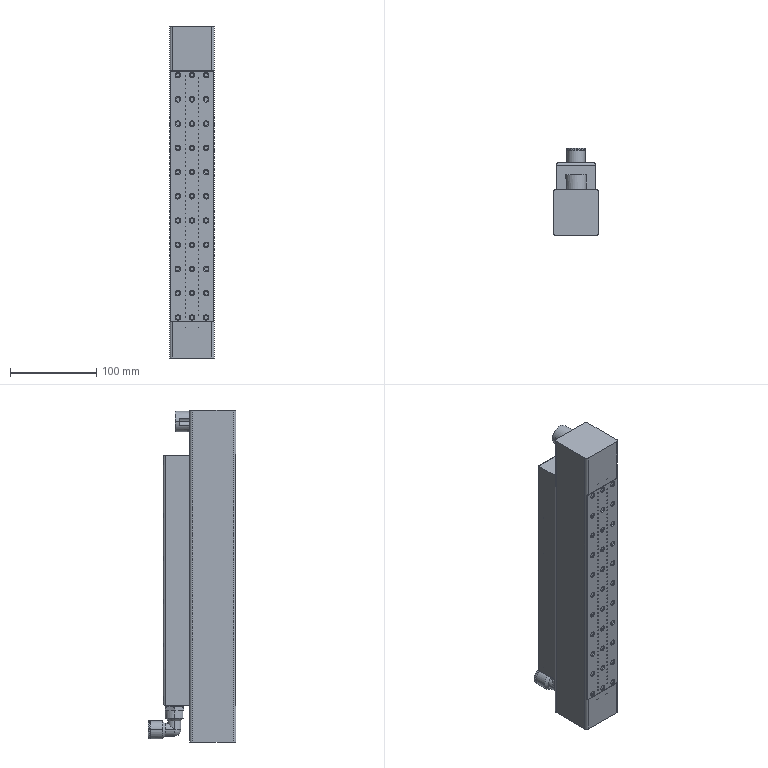Part | SolidWorks | features BaseBody 1 | 1 solid | 920 faces | box 52 x 102 x 385 mm | volume 1482510 mm3 | cylinder 350 | cone 314 | plane 248 | torus 6 | sphere 2 | commonest cylinder face diameters 1 x226 5.3 x24 10 x24 5 x16 6.5 x12 3.2 x8